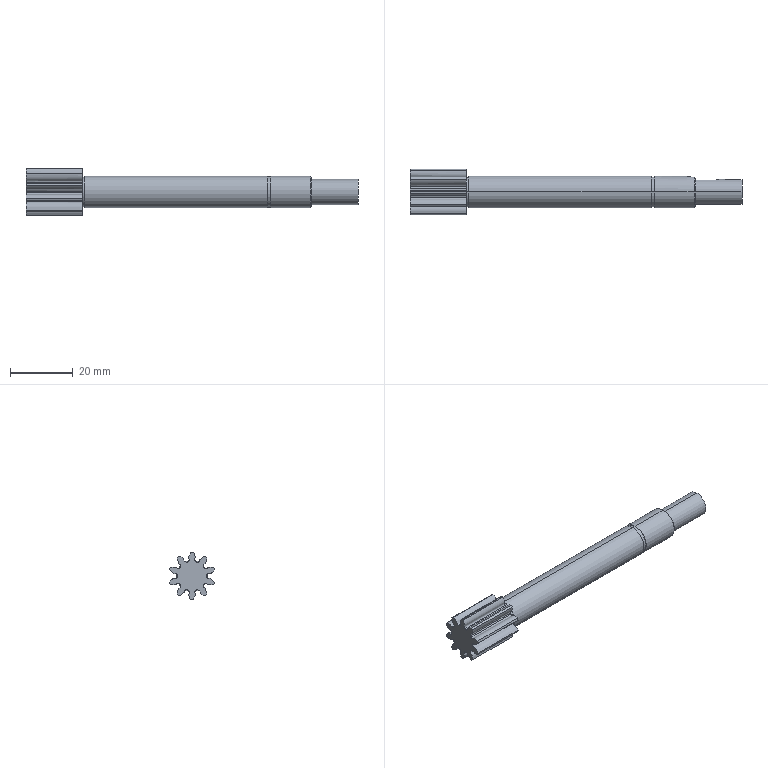Part | SolidWorks | features ICE 7, Chamfer 2, CirPattern 1, Extrusion 1, RefAxis 1 | 1 solid | 86 faces | box 106 x 14.473 x 15 mm | volume 8561 mm3 | cylinder 33 | plane 29 | spline 20 | cone 4 | commonest cylinder face diameters 15 x11 9.375 x10 10 x4 3 x2 8 x2 9.5 x2